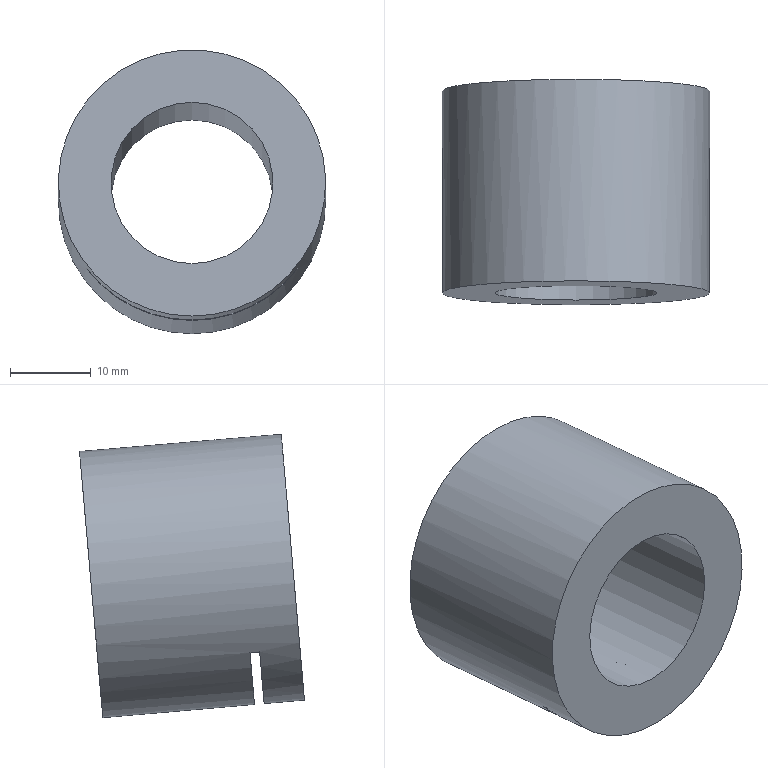Part | NX | features solid 2 | 1 solid | 7 faces | box 33 x 27.781 x 35.053 mm | volume 13389 mm3 | plane 5 | cylinder 2 | commonest cylinder face diameters 20 x1 33 x1
STEP:
#1=CARTESIAN_POINT('',(-462.881,-83.974,-21.096));
#2=VERTEX_POINT('',#1);
#3=CARTESIAN_POINT('',(-462.881,-85.412,-37.533));
#4=DIRECTION('',(0.,0.9962,-0.08716));
#5=DIRECTION('',(0.,0.08716,0.9962));
#6=AXIS2_PLACEMENT_3D('',#3,#4,#5);
#7=CIRCLE('',#6,16.5);
#8=EDGE_CURVE('',#2,#2,#7,.F.);
#9=ORIENTED_EDGE('',*,*,#8,.T.);
#10=EDGE_LOOP('',(#9));
#11=FACE_BOUND('',#10,.T.);
#12=CARTESIAN_POINT('',(-462.881,-111.755,-51.792));
#13=VERTEX_POINT('',#12);
#14=CARTESIAN_POINT('',(-462.881,-110.317,-35.354));
#15=DIRECTION('',(0.,-0.9962,0.08716));
#16=DIRECTION('',(0.,-0.08716,-0.9962));
#17=AXIS2_PLACEMENT_3D('',#14,#15,#16);
#18=CIRCLE('',#17,16.5);
#19=EDGE_CURVE('',#13,#13,#18,.T.);
#20=ORIENTED_EDGE('',*,*,#19,.F.);
#21=EDGE_LOOP('',(#20));
#22=FACE_BOUND('',#21,.T.);
#23=CARTESIAN_POINT('',(-449.833,-106.216,-45.852));
#24=VERTEX_POINT('',#23);
#25=CARTESIAN_POINT('',(-449.833,-105.02,-45.956));
#26=VERTEX_POINT('',#25);
#27=CARTESIAN_POINT('',(-449.833,-69.357,-49.076));
#28=DIRECTION('',(0.,-0.9962,0.08716));
#29=VECTOR('',#28,1000.);
#30=LINE('',#27,#29);
#31=EDGE_CURVE('',#24,#26,#30,.F.);
#32=ORIENTED_EDGE('',*,*,#31,.T.);
#33=CARTESIAN_POINT('',(-475.929,-105.02,-45.956));
#34=VERTEX_POINT('',#33);
#35=CARTESIAN_POINT('',(-462.881,-104.14,-35.895));
#36=DIRECTION('',(0.,-0.9962,0.08716));
#37=DIRECTION('',(0.,-0.08716,-0.9962));
#38=AXIS2_PLACEMENT_3D('',#35,#36,#37);
#39=CIRCLE('',#38,16.5);
#40=EDGE_CURVE('',#26,#34,#39,.F.);
#41=ORIENTED_EDGE('',*,*,#40,.T.);
#42=CARTESIAN_POINT('',(-475.929,-106.216,-45.852));
#43=VERTEX_POINT('',#42);
#44=CARTESIAN_POINT('',(-475.929,-69.357,-49.076));
#45=DIRECTION('',(0.,-0.9962,0.08716));
#46=VECTOR('',#45,1000.);
#47=LINE('',#44,#46);
#48=EDGE_CURVE('',#34,#43,#47,.T.);
#49=ORIENTED_EDGE('',*,*,#48,.T.);
#50=CARTESIAN_POINT('',(-462.881,-105.336,-35.79));
#51=DIRECTION('',(0.,-0.9962,0.08716));
#52=DIRECTION('',(0.,-0.08716,-0.9962));
#53=AXIS2_PLACEMENT_3D('',#50,#51,#52);
#54=CIRCLE('',#53,16.5);
#55=EDGE_CURVE('',#24,#43,#54,.F.);
#56=ORIENTED_EDGE('',*,*,#55,.F.);
#57=EDGE_LOOP('',(#32,#41,#49,#56));
#58=FACE_BOUND('',#57,.T.);
#59=CARTESIAN_POINT('',(-462.881,-76.645,-38.3));
#60=DIRECTION('',(0.,-0.9962,0.08716));
#61=DIRECTION('',(0.,-0.08716,-0.9962));
#62=AXIS2_PLACEMENT_3D('',#59,#60,#61);
#63=CYLINDRICAL_SURFACE('',#62,16.5);
#64=ADVANCED_FACE('',(#11,#22,#58),#63,.T.);
#65=ORIENTED_EDGE('',*,*,#8,.F.);
#66=EDGE_LOOP('',(#65));
#67=FACE_BOUND('',#66,.T.);
#68=CARTESIAN_POINT('',(-462.881,-84.54,-27.571));
#69=VERTEX_POINT('',#68);
#70=CARTESIAN_POINT('',(-462.881,-85.412,-37.533));
#71=DIRECTION('',(0.,0.9962,-0.08716));
#72=DIRECTION('',(0.,0.08716,0.9962));
#73=AXIS2_PLACEMENT_3D('',#70,#71,#72);
#74=CIRCLE('',#73,10.);
#75=EDGE_CURVE('',#69,#69,#74,.F.);
#76=ORIENTED_EDGE('',*,*,#75,.T.);
#77=EDGE_LOOP('',(#76));
#78=FACE_BOUND('',#77,.T.);
#79=CARTESIAN_POINT('',(-462.881,-85.412,-37.533));
#80=DIRECTION('',(0.,0.9962,-0.08716));
#81=DIRECTION('',(-1.,0.,0.));
#82=AXIS2_PLACEMENT_3D('',#79,#80,#81);
#83=PLANE('',#82);
#84=ADVANCED_FACE('',(#67,#78),#83,.T.);
#85=ORIENTED_EDGE('',*,*,#19,.T.);
#86=EDGE_LOOP('',(#85));
#87=FACE_BOUND('',#86,.T.);
#88=CARTESIAN_POINT('',(-462.881,-111.188,-45.316));
#89=VERTEX_POINT('',#88);
#90=CARTESIAN_POINT('',(-462.881,-110.317,-35.354));
#91=DIRECTION('',(0.,-0.9962,0.08716));
#92=DIRECTION('',(0.,-0.08716,-0.9962));
#93=AXIS2_PLACEMENT_3D('',#90,#91,#92);
#94=CIRCLE('',#93,10.);
#95=EDGE_CURVE('',#89,#89,#94,.T.);
#96=ORIENTED_EDGE('',*,*,#95,.F.);
#97=EDGE_LOOP('',(#96));
#98=FACE_BOUND('',#97,.T.);
#99=CARTESIAN_POINT('',(-462.881,-110.317,-35.354));
#100=DIRECTION('',(0.,-0.9962,0.08716));
#101=DIRECTION('',(-1.,0.,0.));
#102=AXIS2_PLACEMENT_3D('',#99,#100,#101);
#103=PLANE('',#102);
#104=ADVANCED_FACE('',(#87,#98),#103,.T.);
#105=ORIENTED_EDGE('',*,*,#75,.F.);
#106=EDGE_LOOP('',(#105));
#107=FACE_BOUND('',#106,.T.);
#108=ORIENTED_EDGE('',*,*,#95,.T.);
#109=EDGE_LOOP('',(#108));
#110=FACE_BOUND('',#109,.T.);
#111=CARTESIAN_POINT('',(-462.881,-62.698,-39.52));
#112=DIRECTION('',(0.,-0.9962,0.08716));
#113=DIRECTION('',(0.,-0.08716,-0.9962));
#114=AXIS2_PLACEMENT_3D('',#111,#112,#113);
#115=CYLINDRICAL_SURFACE('',#114,10.);
#116=ADVANCED_FACE('',(#107,#110),#115,.F.);
#117=CARTESIAN_POINT('',(-476.005,-105.02,-45.956));
#118=DIRECTION('',(-1.,0.,0.));
#119=VECTOR('',#118,1000.);
#120=LINE('',#117,#119);
#121=EDGE_CURVE('',#34,#26,#120,.F.);
#122=ORIENTED_EDGE('',*,*,#121,.F.);
#123=ORIENTED_EDGE('',*,*,#40,.F.);
#124=EDGE_LOOP('',(#122,#123));
#125=FACE_BOUND('',#124,.T.);
#126=CARTESIAN_POINT('',(-476.005,-109.378,-95.766));
#127=DIRECTION('',(0.,-0.9962,0.08716));
#128=DIRECTION('',(0.,-0.08716,-0.9962));
#129=AXIS2_PLACEMENT_3D('',#126,#127,#128);
#130=PLANE('',#129);
#131=ADVANCED_FACE('',(#125),#130,.T.);
#132=ORIENTED_EDGE('',*,*,#55,.T.);
#133=CARTESIAN_POINT('',(-476.005,-106.216,-45.852));
#134=DIRECTION('',(-1.,0.,0.));
#135=VECTOR('',#134,1000.);
#136=LINE('',#133,#135);
#137=EDGE_CURVE('',#43,#24,#136,.F.);
#138=ORIENTED_EDGE('',*,*,#137,.T.);
#139=EDGE_LOOP('',(#132,#138));
#140=FACE_BOUND('',#139,.T.);
#141=CARTESIAN_POINT('',(-476.005,-110.574,-95.661));
#142=DIRECTION('',(0.,-0.9962,0.08716));
#143=DIRECTION('',(0.,-0.08716,-0.9962));
#144=AXIS2_PLACEMENT_3D('',#141,#142,#143);
#145=PLANE('',#144);
#146=ADVANCED_FACE('',(#140),#145,.F.);
#147=ORIENTED_EDGE('',*,*,#121,.T.);
#148=ORIENTED_EDGE('',*,*,#31,.F.);
#149=ORIENTED_EDGE('',*,*,#137,.F.);
#150=ORIENTED_EDGE('',*,*,#48,.F.);
#151=EDGE_LOOP('',(#147,#148,#149,#150));
#152=FACE_BOUND('',#151,.T.);
#153=CARTESIAN_POINT('',(-476.005,-106.216,-45.852));
#154=DIRECTION('',(0.,0.08716,0.9962));
#155=DIRECTION('',(0.,0.9962,-0.08716));
#156=AXIS2_PLACEMENT_3D('',#153,#154,#155);
#157=PLANE('',#156);
#158=ADVANCED_FACE('',(#152),#157,.F.);
#159=CLOSED_SHELL('',(#64,#84,#104,#116,#131,#146,#158));
#160=MANIFOLD_SOLID_BREP('',#159);
#161=(LENGTH_UNIT()NAMED_UNIT(*)SI_UNIT(.MILLI.,.METRE.));
#162=UNCERTAINTY_MEASURE_WITH_UNIT(LENGTH_MEASURE(0.00001),#161,'','');
#163=(NAMED_UNIT(*)PLANE_ANGLE_UNIT()SI_UNIT($,.RADIAN.));
#164=(NAMED_UNIT(*)SI_UNIT($,.STERADIAN.)SOLID_ANGLE_UNIT());
#165=(GEOMETRIC_REPRESENTATION_CONTEXT(3)GLOBAL_UNCERTAINTY_ASSIGNED_CONTEXT((#162))GLOBAL_UNIT_ASSIGNED_CONTEXT((#161,#163,#164))REPRESENTATION_CONTEXT('',''));
#166=ADVANCED_BREP_SHAPE_REPRESENTATION('',(#160),#165);